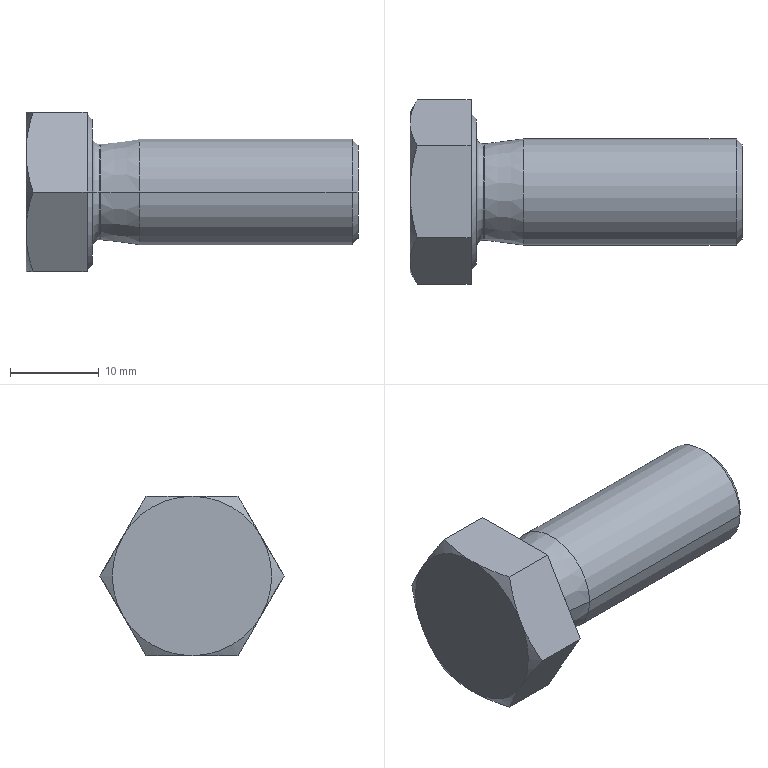Part | SolidWorks | features Chamfer 2, RevCut 2, Revolution 2, Extrusion 1, ICE 1 | 1 solid | 28 faces | box 37.5 x 20.785 x 18 mm | volume 5393 mm3 | cone 12 | plane 10 | torus 4 | cylinder 2 | commonest cylinder face diameters 12 x2
STEP:
#1=CARTESIAN_POINT('',(7.5,-6.282,0.));
#2=VERTEX_POINT('',#1);
#3=CARTESIAN_POINT('',(8.35,-5.432,0.));
#4=VERTEX_POINT('',#3);
#5=CARTESIAN_POINT('',(8.35,-6.282,0.));
#6=DIRECTION('',(0.,0.,-1.));
#7=DIRECTION('',(-1.,0.,0.));
#8=AXIS2_PLACEMENT_3D('',#5,#6,#7);
#9=CIRCLE('',#8,0.85);
#10=EDGE_CURVE('',#2,#4,#9,.T.);
#11=ORIENTED_EDGE('',*,*,#10,.T.);
#12=CARTESIAN_POINT('',(8.35,5.432,0.));
#13=VERTEX_POINT('',#12);
#14=CARTESIAN_POINT('',(8.35,0.,0.));
#15=DIRECTION('',(-1.,0.,0.));
#16=DIRECTION('',(0.,-1.,0.));
#17=AXIS2_PLACEMENT_3D('',#14,#15,#16);
#18=CIRCLE('',#17,5.432);
#19=EDGE_CURVE('',#4,#13,#18,.T.);
#20=ORIENTED_EDGE('',*,*,#19,.T.);
#21=CARTESIAN_POINT('',(7.5,6.282,0.));
#22=VERTEX_POINT('',#21);
#23=CARTESIAN_POINT('',(8.35,6.282,0.));
#24=DIRECTION('',(0.,0.,1.));
#25=DIRECTION('',(0.,-1.,0.));
#26=AXIS2_PLACEMENT_3D('',#23,#24,#25);
#27=CIRCLE('',#26,0.85);
#28=EDGE_CURVE('',#22,#13,#27,.T.);
#29=ORIENTED_EDGE('',*,*,#28,.F.);
#30=CARTESIAN_POINT('',(7.5,0.,0.));
#31=DIRECTION('',(-1.,0.,0.));
#32=DIRECTION('',(0.,-1.,0.));
#33=AXIS2_PLACEMENT_3D('',#30,#31,#32);
#34=CIRCLE('',#33,6.282);
#35=EDGE_CURVE('',#2,#22,#34,.T.);
#36=ORIENTED_EDGE('',*,*,#35,.F.);
#37=EDGE_LOOP('',(#11,#20,#29,#36));
#38=FACE_OUTER_BOUND('',#37,.T.);
#39=CARTESIAN_POINT('',(8.35,0.,0.));
#40=DIRECTION('',(-1.,0.,0.));
#41=DIRECTION('',(0.,-1.,0.));
#42=AXIS2_PLACEMENT_3D('',#39,#40,#41);
#43=TOROIDAL_SURFACE('',#42,6.282,0.85);
#44=ADVANCED_FACE('',(#38),#43,.F.);
#45=ORIENTED_EDGE('',*,*,#28,.T.);
#46=CARTESIAN_POINT('',(8.35,0.,0.));
#47=DIRECTION('',(-1.,0.,0.));
#48=DIRECTION('',(0.,-1.,0.));
#49=AXIS2_PLACEMENT_3D('',#46,#47,#48);
#50=CIRCLE('',#49,5.432);
#51=EDGE_CURVE('',#13,#4,#50,.T.);
#52=ORIENTED_EDGE('',*,*,#51,.T.);
#53=ORIENTED_EDGE('',*,*,#10,.F.);
#54=CARTESIAN_POINT('',(7.5,0.,0.));
#55=DIRECTION('',(-1.,0.,0.));
#56=DIRECTION('',(0.,-1.,0.));
#57=AXIS2_PLACEMENT_3D('',#54,#55,#56);
#58=CIRCLE('',#57,6.282);
#59=EDGE_CURVE('',#22,#2,#58,.T.);
#60=ORIENTED_EDGE('',*,*,#59,.F.);
#61=EDGE_LOOP('',(#45,#52,#53,#60));
#62=FACE_OUTER_BOUND('',#61,.T.);
#63=CARTESIAN_POINT('',(8.35,0.,0.));
#64=DIRECTION('',(-1.,0.,0.));
#65=DIRECTION('',(0.,-1.,0.));
#66=AXIS2_PLACEMENT_3D('',#63,#64,#65);
#67=TOROIDAL_SURFACE('',#66,6.282,0.85);
#68=ADVANCED_FACE('',(#62),#67,.F.);
#69=CARTESIAN_POINT('',(7.5,-8.215,0.));
#70=VERTEX_POINT('',#69);
#71=CARTESIAN_POINT('',(7.5,8.215,0.));
#72=VERTEX_POINT('',#71);
#73=CARTESIAN_POINT('',(7.5,0.,0.));
#74=DIRECTION('',(-1.,0.,0.));
#75=DIRECTION('',(0.,-1.,0.));
#76=AXIS2_PLACEMENT_3D('',#73,#74,#75);
#77=CIRCLE('',#76,8.215);
#78=EDGE_CURVE('',#70,#72,#77,.T.);
#79=ORIENTED_EDGE('',*,*,#78,.T.);
#80=CARTESIAN_POINT('',(6.9,8.815,0.));
#81=VERTEX_POINT('',#80);
#82=CARTESIAN_POINT('',(6.9,8.815,0.));
#83=DIRECTION('',(-0.7071,0.7071,0.));
#84=VECTOR('',#83,1000.);
#85=LINE('',#82,#84);
#86=EDGE_CURVE('',#72,#81,#85,.T.);
#87=ORIENTED_EDGE('',*,*,#86,.T.);
#88=CARTESIAN_POINT('',(6.9,-8.815,0.));
#89=VERTEX_POINT('',#88);
#90=CARTESIAN_POINT('',(6.9,0.,0.));
#91=DIRECTION('',(-1.,0.,0.));
#92=DIRECTION('',(0.,-1.,0.));
#93=AXIS2_PLACEMENT_3D('',#90,#91,#92);
#94=CIRCLE('',#93,8.815);
#95=EDGE_CURVE('',#89,#81,#94,.T.);
#96=ORIENTED_EDGE('',*,*,#95,.F.);
#97=CARTESIAN_POINT('',(6.9,-8.815,0.));
#98=DIRECTION('',(-0.7071,-0.7071,0.));
#99=VECTOR('',#98,1000.);
#100=LINE('',#97,#99);
#101=EDGE_CURVE('',#70,#89,#100,.T.);
#102=ORIENTED_EDGE('',*,*,#101,.F.);
#103=EDGE_LOOP('',(#79,#87,#96,#102));
#104=FACE_OUTER_BOUND('',#103,.T.);
#105=CARTESIAN_POINT('',(6.9,0.,0.));
#106=DIRECTION('',(-1.,0.,0.));
#107=DIRECTION('',(0.,-1.,0.));
#108=AXIS2_PLACEMENT_3D('',#105,#106,#107);
#109=CONICAL_SURFACE('',#108,8.815,0.7854);
#110=ADVANCED_FACE('',(#104),#109,.T.);
#111=CARTESIAN_POINT('',(37.5,5.333,0.));
#112=VERTEX_POINT('',#111);
#113=CARTESIAN_POINT('',(37.5,-5.333,0.));
#114=VERTEX_POINT('',#113);
#115=CARTESIAN_POINT('',(37.5,0.,0.));
#116=DIRECTION('',(1.,0.,0.));
#117=DIRECTION('',(0.,-1.,0.));
#118=AXIS2_PLACEMENT_3D('',#115,#116,#117);
#119=CIRCLE('',#118,5.333);
#120=EDGE_CURVE('',#112,#114,#119,.T.);
#121=ORIENTED_EDGE('',*,*,#120,.F.);
#122=CARTESIAN_POINT('',(36.833,6.,0.));
#123=VERTEX_POINT('',#122);
#124=CARTESIAN_POINT('',(36.833,6.,0.));
#125=DIRECTION('',(-0.7071,0.7071,0.));
#126=VECTOR('',#125,1000.);
#127=LINE('',#124,#126);
#128=EDGE_CURVE('',#112,#123,#127,.T.);
#129=ORIENTED_EDGE('',*,*,#128,.T.);
#130=CARTESIAN_POINT('',(36.833,-6.,0.));
#131=VERTEX_POINT('',#130);
#132=CARTESIAN_POINT('',(36.833,0.,0.));
#133=DIRECTION('',(-1.,0.,0.));
#134=DIRECTION('',(0.,-1.,0.));
#135=AXIS2_PLACEMENT_3D('',#132,#133,#134);
#136=CIRCLE('',#135,6.);
#137=EDGE_CURVE('',#131,#123,#136,.T.);
#138=ORIENTED_EDGE('',*,*,#137,.F.);
#139=CARTESIAN_POINT('',(36.833,-6.,0.));
#140=DIRECTION('',(-0.7071,-0.7071,0.));
#141=VECTOR('',#140,1000.);
#142=LINE('',#139,#141);
#143=EDGE_CURVE('',#114,#131,#142,.T.);
#144=ORIENTED_EDGE('',*,*,#143,.F.);
#145=EDGE_LOOP('',(#121,#129,#138,#144));
#146=FACE_OUTER_BOUND('',#145,.T.);
#147=CARTESIAN_POINT('',(36.833,0.,0.));
#148=DIRECTION('',(-1.,0.,0.));
#149=DIRECTION('',(0.,-1.,0.));
#150=AXIS2_PLACEMENT_3D('',#147,#148,#149);
#151=CONICAL_SURFACE('',#150,6.,0.7854);
#152=ADVANCED_FACE('',(#146),#151,.T.);
#153=ORIENTED_EDGE('',*,*,#51,.F.);
#154=CARTESIAN_POINT('',(8.459,5.439,0.));
#155=VERTEX_POINT('',#154);
#156=CARTESIAN_POINT('',(8.35,6.282,0.));
#157=DIRECTION('',(0.,0.,1.));
#158=DIRECTION('',(0.,-1.,0.));
#159=AXIS2_PLACEMENT_3D('',#156,#157,#158);
#160=CIRCLE('',#159,0.85);
#161=EDGE_CURVE('',#13,#155,#160,.T.);
#162=ORIENTED_EDGE('',*,*,#161,.T.);
#163=CARTESIAN_POINT('',(8.459,-5.439,0.));
#164=VERTEX_POINT('',#163);
#165=CARTESIAN_POINT('',(8.459,0.,0.));
#166=DIRECTION('',(-1.,0.,0.));
#167=DIRECTION('',(0.,-1.,0.));
#168=AXIS2_PLACEMENT_3D('',#165,#166,#167);
#169=CIRCLE('',#168,5.439);
#170=EDGE_CURVE('',#155,#164,#169,.T.);
#171=ORIENTED_EDGE('',*,*,#170,.T.);
#172=CARTESIAN_POINT('',(8.35,-6.282,0.));
#173=DIRECTION('',(0.,0.,-1.));
#174=DIRECTION('',(-1.,0.,0.));
#175=AXIS2_PLACEMENT_3D('',#172,#173,#174);
#176=CIRCLE('',#175,0.85);
#177=EDGE_CURVE('',#4,#164,#176,.T.);
#178=ORIENTED_EDGE('',*,*,#177,.F.);
#179=EDGE_LOOP('',(#153,#162,#171,#178));
#180=FACE_OUTER_BOUND('',#179,.T.);
#181=CARTESIAN_POINT('',(8.35,0.,0.));
#182=DIRECTION('',(-1.,0.,0.));
#183=DIRECTION('',(0.,-1.,0.));
#184=AXIS2_PLACEMENT_3D('',#181,#182,#183);
#185=TOROIDAL_SURFACE('',#184,6.282,0.85);
#186=ADVANCED_FACE('',(#180),#185,.F.);
#187=ORIENTED_EDGE('',*,*,#137,.T.);
#188=CARTESIAN_POINT('',(12.8,6.,0.));
#189=VERTEX_POINT('',#188);
#190=CARTESIAN_POINT('',(7.5,6.,0.));
#191=DIRECTION('',(-1.,0.,0.));
#192=VECTOR('',#191,1000.);
#193=LINE('',#190,#192);
#194=EDGE_CURVE('',#123,#189,#193,.T.);
#195=ORIENTED_EDGE('',*,*,#194,.T.);
#196=CARTESIAN_POINT('',(12.8,-6.,0.));
#197=VERTEX_POINT('',#196);
#198=CARTESIAN_POINT('',(12.8,0.,0.));
#199=DIRECTION('',(-1.,0.,0.));
#200=DIRECTION('',(0.,-1.,0.));
#201=AXIS2_PLACEMENT_3D('',#198,#199,#200);
#202=CIRCLE('',#201,6.);
#203=EDGE_CURVE('',#197,#189,#202,.T.);
#204=ORIENTED_EDGE('',*,*,#203,.F.);
#205=CARTESIAN_POINT('',(7.5,-6.,0.));
#206=DIRECTION('',(-1.,0.,0.));
#207=VECTOR('',#206,1000.);
#208=LINE('',#205,#207);
#209=EDGE_CURVE('',#131,#197,#208,.T.);
#210=ORIENTED_EDGE('',*,*,#209,.F.);
#211=EDGE_LOOP('',(#187,#195,#204,#210));
#212=FACE_OUTER_BOUND('',#211,.T.);
#213=CARTESIAN_POINT('',(7.5,0.,0.));
#214=DIRECTION('',(-1.,0.,0.));
#215=DIRECTION('',(0.,-1.,0.));
#216=AXIS2_PLACEMENT_3D('',#213,#214,#215);
#217=CYLINDRICAL_SURFACE('',#216,6.);
#218=ADVANCED_FACE('',(#212),#217,.T.);
#219=CARTESIAN_POINT('',(8.459,0.,0.));
#220=DIRECTION('',(-1.,0.,0.));
#221=DIRECTION('',(0.,-1.,0.));
#222=AXIS2_PLACEMENT_3D('',#219,#220,#221);
#223=CIRCLE('',#222,5.439);
#224=EDGE_CURVE('',#164,#155,#223,.T.);
#225=ORIENTED_EDGE('',*,*,#224,.F.);
#226=CARTESIAN_POINT('',(12.8,-6.,0.));
#227=DIRECTION('',(0.9917,-0.1282,0.));
#228=VECTOR('',#227,1000.);
#229=LINE('',#226,#228);
#230=EDGE_CURVE('',#164,#197,#229,.T.);
#231=ORIENTED_EDGE('',*,*,#230,.T.);
#232=ORIENTED_EDGE('',*,*,#203,.T.);
#233=CARTESIAN_POINT('',(12.8,6.,0.));
#234=DIRECTION('',(0.9917,0.1282,0.));
#235=VECTOR('',#234,1000.);
#236=LINE('',#233,#235);
#237=EDGE_CURVE('',#155,#189,#236,.T.);
#238=ORIENTED_EDGE('',*,*,#237,.F.);
#239=EDGE_LOOP('',(#225,#231,#232,#238));
#240=FACE_OUTER_BOUND('',#239,.T.);
#241=CARTESIAN_POINT('',(12.8,0.,0.));
#242=DIRECTION('',(1.,0.,0.));
#243=DIRECTION('',(0.,1.,0.));
#244=AXIS2_PLACEMENT_3D('',#241,#242,#243);
#245=CONICAL_SURFACE('',#244,6.,0.1286);
#246=ADVANCED_FACE('',(#240),#245,.T.);
#247=ORIENTED_EDGE('',*,*,#35,.T.);
#248=ORIENTED_EDGE('',*,*,#59,.T.);
#249=EDGE_LOOP('',(#247,#248));
#250=FACE_BOUND('',#249,.T.);
#251=ORIENTED_EDGE('',*,*,#78,.F.);
#252=CARTESIAN_POINT('',(7.5,0.,0.));
#253=DIRECTION('',(-1.,0.,0.));
#254=DIRECTION('',(0.,-1.,0.));
#255=AXIS2_PLACEMENT_3D('',#252,#253,#254);
#256=CIRCLE('',#255,8.215);
#257=EDGE_CURVE('',#72,#70,#256,.T.);
#258=ORIENTED_EDGE('',*,*,#257,.F.);
#259=EDGE_LOOP('',(#251,#258));
#260=FACE_OUTER_BOUND('',#259,.T.);
#261=CARTESIAN_POINT('',(7.5,5.196,-9.));
#262=DIRECTION('',(1.,0.,0.));
#263=DIRECTION('',(0.,0.,-1.));
#264=AXIS2_PLACEMENT_3D('',#261,#262,#263);
#265=PLANE('',#264);
#266=ADVANCED_FACE('',(#250,#260),#265,.T.);
#267=ORIENTED_EDGE('',*,*,#230,.F.);
#268=ORIENTED_EDGE('',*,*,#170,.F.);
#269=ORIENTED_EDGE('',*,*,#237,.T.);
#270=CARTESIAN_POINT('',(12.8,0.,0.));
#271=DIRECTION('',(-1.,0.,0.));
#272=DIRECTION('',(0.,-1.,0.));
#273=AXIS2_PLACEMENT_3D('',#270,#271,#272);
#274=CIRCLE('',#273,6.);
#275=EDGE_CURVE('',#189,#197,#274,.T.);
#276=ORIENTED_EDGE('',*,*,#275,.T.);
#277=EDGE_LOOP('',(#267,#268,#269,#276));
#278=FACE_OUTER_BOUND('',#277,.T.);
#279=CARTESIAN_POINT('',(12.8,0.,0.));
#280=DIRECTION('',(1.,0.,0.));
#281=DIRECTION('',(0.,1.,0.));
#282=AXIS2_PLACEMENT_3D('',#279,#280,#281);
#283=CONICAL_SURFACE('',#282,6.,0.1286);
#284=ADVANCED_FACE('',(#278),#283,.T.);
#285=ORIENTED_EDGE('',*,*,#194,.F.);
#286=CARTESIAN_POINT('',(36.833,0.,0.));
#287=DIRECTION('',(-1.,0.,0.));
#288=DIRECTION('',(0.,-1.,0.));
#289=AXIS2_PLACEMENT_3D('',#286,#287,#288);
#290=CIRCLE('',#289,6.);
#291=EDGE_CURVE('',#123,#131,#290,.T.);
#292=ORIENTED_EDGE('',*,*,#291,.T.);
#293=ORIENTED_EDGE('',*,*,#209,.T.);
#294=ORIENTED_EDGE('',*,*,#275,.F.);
#295=EDGE_LOOP('',(#285,#292,#293,#294));
#296=FACE_OUTER_BOUND('',#295,.T.);
#297=CARTESIAN_POINT('',(7.5,0.,0.));
#298=DIRECTION('',(-1.,0.,0.));
#299=DIRECTION('',(0.,-1.,0.));
#300=AXIS2_PLACEMENT_3D('',#297,#298,#299);
#301=CYLINDRICAL_SURFACE('',#300,6.);
#302=ADVANCED_FACE('',(#296),#301,.T.);
#303=CARTESIAN_POINT('',(37.5,0.,0.));
#304=DIRECTION('',(1.,0.,0.));
#305=DIRECTION('',(0.,-1.,0.));
#306=AXIS2_PLACEMENT_3D('',#303,#304,#305);
#307=CIRCLE('',#306,5.333);
#308=EDGE_CURVE('',#114,#112,#307,.T.);
#309=ORIENTED_EDGE('',*,*,#308,.T.);
#310=ORIENTED_EDGE('',*,*,#120,.T.);
#311=EDGE_LOOP('',(#309,#310));
#312=FACE_OUTER_BOUND('',#311,.T.);
#313=CARTESIAN_POINT('',(37.5,6.,0.));
#314=DIRECTION('',(-1.,0.,0.));
#315=DIRECTION('',(0.,-1.,0.));
#316=AXIS2_PLACEMENT_3D('',#313,#314,#315);
#317=PLANE('',#316);
#318=ADVANCED_FACE('',(#312),#317,.F.);
#319=ORIENTED_EDGE('',*,*,#19,.F.);
#320=ORIENTED_EDGE('',*,*,#177,.T.);
#321=ORIENTED_EDGE('',*,*,#224,.T.);
#322=ORIENTED_EDGE('',*,*,#161,.F.);
#323=EDGE_LOOP('',(#319,#320,#321,#322));
#324=FACE_OUTER_BOUND('',#323,.T.);
#325=CARTESIAN_POINT('',(8.35,0.,0.));
#326=DIRECTION('',(-1.,0.,0.));
#327=DIRECTION('',(0.,-1.,0.));
#328=AXIS2_PLACEMENT_3D('',#325,#326,#327);
#329=TOROIDAL_SURFACE('',#328,6.282,0.85);
#330=ADVANCED_FACE('',(#324),#329,.F.);
#331=ORIENTED_EDGE('',*,*,#128,.F.);
#332=ORIENTED_EDGE('',*,*,#308,.F.);
#333=ORIENTED_EDGE('',*,*,#143,.T.);
#334=ORIENTED_EDGE('',*,*,#291,.F.);
#335=EDGE_LOOP('',(#331,#332,#333,#334));
#336=FACE_OUTER_BOUND('',#335,.T.);
#337=CARTESIAN_POINT('',(36.833,0.,0.));
#338=DIRECTION('',(-1.,0.,0.));
#339=DIRECTION('',(0.,-1.,0.));
#340=AXIS2_PLACEMENT_3D('',#337,#338,#339);
#341=CONICAL_SURFACE('',#340,6.,0.7854);
#342=ADVANCED_FACE('',(#336),#341,.T.);
#343=ORIENTED_EDGE('',*,*,#95,.T.);
#344=CARTESIAN_POINT('',(6.9,0.,0.));
#345=DIRECTION('',(-1.,0.,0.));
#346=DIRECTION('',(0.,-1.,0.));
#347=AXIS2_PLACEMENT_3D('',#344,#345,#346);
#348=CIRCLE('',#347,8.815);
#349=EDGE_CURVE('',#81,#89,#348,.T.);
#350=ORIENTED_EDGE('',*,*,#349,.T.);
#351=EDGE_LOOP('',(#343,#350));
#352=FACE_BOUND('',#351,.T.);
#353=CARTESIAN_POINT('',(6.9,-5.196,-9.));
#354=VERTEX_POINT('',#353);
#355=CARTESIAN_POINT('',(6.9,5.196,-9.));
#356=VERTEX_POINT('',#355);
#357=CARTESIAN_POINT('',(6.9,-5.196,-9.));
#358=DIRECTION('',(0.,1.,0.));
#359=VECTOR('',#358,1000.);
#360=LINE('',#357,#359);
#361=EDGE_CURVE('',#354,#356,#360,.T.);
#362=ORIENTED_EDGE('',*,*,#361,.T.);
#363=CARTESIAN_POINT('',(6.9,10.392,0.));
#364=VERTEX_POINT('',#363);
#365=CARTESIAN_POINT('',(6.9,5.196,-9.));
#366=DIRECTION('',(0.,0.5,0.866));
#367=VECTOR('',#366,1000.);
#368=LINE('',#365,#367);
#369=EDGE_CURVE('',#356,#364,#368,.T.);
#370=ORIENTED_EDGE('',*,*,#369,.T.);
#371=CARTESIAN_POINT('',(6.9,5.196,9.));
#372=VERTEX_POINT('',#371);
#373=CARTESIAN_POINT('',(6.9,10.392,0.));
#374=DIRECTION('',(0.,-0.5,0.866));
#375=VECTOR('',#374,1000.);
#376=LINE('',#373,#375);
#377=EDGE_CURVE('',#364,#372,#376,.T.);
#378=ORIENTED_EDGE('',*,*,#377,.T.);
#379=CARTESIAN_POINT('',(6.9,-5.196,9.));
#380=VERTEX_POINT('',#379);
#381=CARTESIAN_POINT('',(6.9,5.196,9.));
#382=DIRECTION('',(0.,-1.,0.));
#383=VECTOR('',#382,1000.);
#384=LINE('',#381,#383);
#385=EDGE_CURVE('',#372,#380,#384,.T.);
#386=ORIENTED_EDGE('',*,*,#385,.T.);
#387=CARTESIAN_POINT('',(6.9,-10.392,0.));
#388=VERTEX_POINT('',#387);
#389=CARTESIAN_POINT('',(6.9,-5.196,9.));
#390=DIRECTION('',(0.,-0.5,-0.866));
#391=VECTOR('',#390,1000.);
#392=LINE('',#389,#391);
#393=EDGE_CURVE('',#380,#388,#392,.T.);
#394=ORIENTED_EDGE('',*,*,#393,.T.);
#395=CARTESIAN_POINT('',(6.9,-10.392,0.));
#396=DIRECTION('',(0.,0.5,-0.866));
#397=VECTOR('',#396,1000.);
#398=LINE('',#395,#397);
#399=EDGE_CURVE('',#388,#354,#398,.T.);
#400=ORIENTED_EDGE('',*,*,#399,.T.);
#401=EDGE_LOOP('',(#362,#370,#378,#386,#394,#400));
#402=FACE_OUTER_BOUND('',#401,.T.);
#403=CARTESIAN_POINT('',(6.9,-8.815,0.));
#404=DIRECTION('',(1.,0.,0.));
#405=DIRECTION('',(0.,1.,0.));
#406=AXIS2_PLACEMENT_3D('',#403,#404,#405);
#407=PLANE('',#406);
#408=ADVANCED_FACE('',(#352,#402),#407,.T.);
#409=ORIENTED_EDGE('',*,*,#86,.F.);
#410=ORIENTED_EDGE('',*,*,#257,.T.);
#411=ORIENTED_EDGE('',*,*,#101,.T.);
#412=ORIENTED_EDGE('',*,*,#349,.F.);
#413=EDGE_LOOP('',(#409,#410,#411,#412));
#414=FACE_OUTER_BOUND('',#413,.T.);
#415=CARTESIAN_POINT('',(6.9,0.,0.));
#416=DIRECTION('',(-1.,0.,0.));
#417=DIRECTION('',(0.,-1.,0.));
#418=AXIS2_PLACEMENT_3D('',#415,#416,#417);
#419=CONICAL_SURFACE('',#418,8.815,0.7854);
#420=ADVANCED_FACE('',(#414),#419,.T.);
#421=CARTESIAN_POINT('',(0.,0.,-9.));
#422=VERTEX_POINT('',#421);
#423=CARTESIAN_POINT('',(0.,7.794,-4.5));
#424=VERTEX_POINT('',#423);
#425=CARTESIAN_POINT('',(0.,0.,0.));
#426=DIRECTION('',(1.,0.,0.));
#427=DIRECTION('',(0.,0.,-1.));
#428=AXIS2_PLACEMENT_3D('',#425,#426,#427);
#429=CIRCLE('',#428,9.);
#430=EDGE_CURVE('',#422,#424,#429,.T.);
#431=ORIENTED_EDGE('',*,*,#430,.F.);
#432=CARTESIAN_POINT('',(0.,-7.794,-4.5));
#433=VERTEX_POINT('',#432);
#434=CARTESIAN_POINT('',(0.,0.,0.));
#435=DIRECTION('',(1.,0.,0.));
#436=DIRECTION('',(0.,0.,-1.));
#437=AXIS2_PLACEMENT_3D('',#434,#435,#436);
#438=CIRCLE('',#437,9.);
#439=EDGE_CURVE('',#433,#422,#438,.T.);
#440=ORIENTED_EDGE('',*,*,#439,.F.);
#441=CARTESIAN_POINT('',(0.,-7.794,4.5));
#442=VERTEX_POINT('',#441);
#443=CARTESIAN_POINT('',(0.,0.,0.));
#444=DIRECTION('',(1.,0.,0.));
#445=DIRECTION('',(0.,0.,-1.));
#446=AXIS2_PLACEMENT_3D('',#443,#444,#445);
#447=CIRCLE('',#446,9.);
#448=EDGE_CURVE('',#442,#433,#447,.T.);
#449=ORIENTED_EDGE('',*,*,#448,.F.);
#450=CARTESIAN_POINT('',(0.,0.,9.));
#451=VERTEX_POINT('',#450);
#452=CARTESIAN_POINT('',(0.,0.,0.));
#453=DIRECTION('',(1.,0.,0.));
#454=DIRECTION('',(0.,0.,-1.));
#455=AXIS2_PLACEMENT_3D('',#452,#453,#454);
#456=CIRCLE('',#455,9.);
#457=EDGE_CURVE('',#451,#442,#456,.T.);
#458=ORIENTED_EDGE('',*,*,#457,.F.);
#459=CARTESIAN_POINT('',(0.,7.794,4.5));
#460=VERTEX_POINT('',#459);
#461=CARTESIAN_POINT('',(0.,0.,0.));
#462=DIRECTION('',(-1.,0.,0.));
#463=DIRECTION('',(0.,0.,1.));
#464=AXIS2_PLACEMENT_3D('',#461,#462,#463);
#465=CIRCLE('',#464,9.);
#466=EDGE_CURVE('',#451,#460,#465,.T.);
#467=ORIENTED_EDGE('',*,*,#466,.T.);
#468=CARTESIAN_POINT('',(0.,0.,0.));
#469=DIRECTION('',(1.,0.,0.));
#470=DIRECTION('',(0.,0.,-1.));
#471=AXIS2_PLACEMENT_3D('',#468,#469,#470);
#472=CIRCLE('',#471,9.);
#473=EDGE_CURVE('',#424,#460,#472,.T.);
#474=ORIENTED_EDGE('',*,*,#473,.F.);
#475=EDGE_LOOP('',(#431,#440,#449,#458,#467,#474));
#476=FACE_OUTER_BOUND('',#475,.T.);
#477=CARTESIAN_POINT('',(0.,5.196,-9.));
#478=DIRECTION('',(1.,0.,0.));
#479=DIRECTION('',(0.,0.,-1.));
#480=AXIS2_PLACEMENT_3D('',#477,#478,#479);
#481=PLANE('',#480);
#482=ADVANCED_FACE('',(#476),#481,.F.);
#483=CARTESIAN_POINT('',(0.8038,5.196,-9.));
#484=VERTEX_POINT('',#483);
#485=CARTESIAN_POINT('',(0.,7.794,-4.5));
#486=CARTESIAN_POINT('',(0.,7.574,-4.882));
#487=CARTESIAN_POINT('',(0.019,7.352,-5.266));
#488=CARTESIAN_POINT('',(0.09253,6.914,-6.024));
#489=CARTESIAN_POINT('',(0.147,6.697,-6.401));
#490=CARTESIAN_POINT('',(0.357,6.048,-7.525));
#491=CARTESIAN_POINT('',(0.5591,5.62,-8.266));
#492=CARTESIAN_POINT('',(0.8038,5.196,-9.));
#493=B_SPLINE_CURVE_WITH_KNOTS('',3,(#485,#486,#487,#488,#489,#490,#491,#492),.UNSPECIFIED.,.F.,.F.,(4,2,2,4),(0.005258,0.006567,0.007877,0.0105),.UNSPECIFIED.);
#494=EDGE_CURVE('',#424,#484,#493,.T.);
#495=ORIENTED_EDGE('',*,*,#494,.T.);
#496=CARTESIAN_POINT('',(0.8038,5.196,-9.));
#497=CARTESIAN_POINT('',(0.5613,4.356,-9.));
#498=CARTESIAN_POINT('',(0.3593,3.505,-9.));
#499=CARTESIAN_POINT('',(0.07758,1.769,-9.));
#500=CARTESIAN_POINT('',(0.,0.8787,-9.));
#501=CARTESIAN_POINT('',(0.,0.,-9.));
#502=B_SPLINE_CURVE_WITH_KNOTS('',3,(#496,#497,#498,#499,#500,#501),.UNSPECIFIED.,.F.,.F.,(4,2,4),(0.003787,0.00641,0.009033),.UNSPECIFIED.);
#503=EDGE_CURVE('',#484,#422,#502,.T.);
#504=ORIENTED_EDGE('',*,*,#503,.T.);
#505=ORIENTED_EDGE('',*,*,#430,.T.);
#506=EDGE_LOOP('',(#495,#504,#505));
#507=FACE_OUTER_BOUND('',#506,.T.);
#508=CARTESIAN_POINT('',(0.,0.,0.));
#509=DIRECTION('',(1.,0.,0.));
#510=DIRECTION('',(0.,0.,1.));
#511=AXIS2_PLACEMENT_3D('',#508,#509,#510);
#512=CONICAL_SURFACE('',#511,9.,1.047);
#513=ADVANCED_FACE('',(#507),#512,.T.);
#514=CARTESIAN_POINT('',(0.8038,10.392,0.));
#515=VERTEX_POINT('',#514);
#516=CARTESIAN_POINT('',(0.,7.794,4.5));
#517=CARTESIAN_POINT('',(0.,8.015,4.118));
#518=CARTESIAN_POINT('',(0.019,8.236,3.734));
#519=CARTESIAN_POINT('',(0.09253,8.674,2.976));
#520=CARTESIAN_POINT('',(0.147,8.892,2.599));
#521=CARTESIAN_POINT('',(0.357,9.541,1.475));
#522=CARTESIAN_POINT('',(0.5591,9.968,0.7343));
#523=CARTESIAN_POINT('',(0.8038,10.392,0.));
#524=B_SPLINE_CURVE_WITH_KNOTS('',3,(#516,#517,#518,#519,#520,#521,#522,#523),.UNSPECIFIED.,.F.,.F.,(4,2,2,4),(0.005258,0.006567,0.007877,0.0105),.UNSPECIFIED.);
#525=EDGE_CURVE('',#460,#515,#524,.T.);
#526=ORIENTED_EDGE('',*,*,#525,.T.);
#527=CARTESIAN_POINT('',(0.8038,10.392,0.));
#528=CARTESIAN_POINT('',(0.5585,9.967,-0.7361));
#529=CARTESIAN_POINT('',(0.3563,9.539,-1.478));
#530=CARTESIAN_POINT('',(0.07661,8.674,-2.976));
#531=CARTESIAN_POINT('',(0.,8.237,-3.733));
#532=CARTESIAN_POINT('',(0.,7.794,-4.5));
#533=B_SPLINE_CURVE_WITH_KNOTS('',3,(#527,#528,#529,#530,#531,#532),.UNSPECIFIED.,.F.,.F.,(4,2,4),(0.000000238,0.002629,0.005258),.UNSPECIFIED.);
#534=EDGE_CURVE('',#515,#424,#533,.T.);
#535=ORIENTED_EDGE('',*,*,#534,.T.);
#536=ORIENTED_EDGE('',*,*,#473,.T.);
#537=EDGE_LOOP('',(#526,#535,#536));
#538=FACE_OUTER_BOUND('',#537,.T.);
#539=CARTESIAN_POINT('',(0.,0.,0.));
#540=DIRECTION('',(1.,0.,0.));
#541=DIRECTION('',(0.,0.,1.));
#542=AXIS2_PLACEMENT_3D('',#539,#540,#541);
#543=CONICAL_SURFACE('',#542,9.,1.047);
#544=ADVANCED_FACE('',(#538),#543,.T.);
#545=CARTESIAN_POINT('',(0.8038,5.196,9.));
#546=VERTEX_POINT('',#545);
#547=CARTESIAN_POINT('',(0.8038,5.196,9.));
#548=CARTESIAN_POINT('',(0.5585,5.621,8.264));
#549=CARTESIAN_POINT('',(0.3563,6.049,7.522));
#550=CARTESIAN_POINT('',(0.07661,6.914,6.024));
#551=CARTESIAN_POINT('',(0.,7.352,5.267));
#552=CARTESIAN_POINT('',(0.,7.794,4.5));
#553=B_SPLINE_CURVE_WITH_KNOTS('',3,(#547,#548,#549,#550,#551,#552),.UNSPECIFIED.,.F.,.F.,(4,2,4),(0.000000238,0.002629,0.005258),.UNSPECIFIED.);
#554=EDGE_CURVE('',#546,#460,#553,.T.);
#555=ORIENTED_EDGE('',*,*,#554,.T.);
#556=ORIENTED_EDGE('',*,*,#466,.F.);
#557=CARTESIAN_POINT('',(0.,0.,9.));
#558=CARTESIAN_POINT('',(0.,0.8787,9.));
#559=CARTESIAN_POINT('',(0.07758,1.769,9.));
#560=CARTESIAN_POINT('',(0.3593,3.505,9.));
#561=CARTESIAN_POINT('',(0.5613,4.356,9.));
#562=CARTESIAN_POINT('',(0.8038,5.196,9.));
#563=B_SPLINE_CURVE_WITH_KNOTS('',3,(#557,#558,#559,#560,#561,#562),.UNSPECIFIED.,.F.,.F.,(4,2,4),(0.01455,0.01718,0.01981),.UNSPECIFIED.);
#564=EDGE_CURVE('',#451,#546,#563,.T.);
#565=ORIENTED_EDGE('',*,*,#564,.T.);
#566=EDGE_LOOP('',(#555,#556,#565));
#567=FACE_OUTER_BOUND('',#566,.T.);
#568=CARTESIAN_POINT('',(0.,0.,0.));
#569=DIRECTION('',(1.,0.,0.));
#570=DIRECTION('',(0.,0.,1.));
#571=AXIS2_PLACEMENT_3D('',#568,#569,#570);
#572=CONICAL_SURFACE('',#571,9.,1.047);
#573=ADVANCED_FACE('',(#567),#572,.T.);
#574=CARTESIAN_POINT('',(0.8038,-5.196,9.));
#575=VERTEX_POINT('',#574);
#576=CARTESIAN_POINT('',(0.8038,-5.196,9.));
#577=CARTESIAN_POINT('',(0.5599,-4.351,9.));
#578=CARTESIAN_POINT('',(0.3553,-3.485,9.));
#579=CARTESIAN_POINT('',(0.07548,-1.75,9.));
#580=CARTESIAN_POINT('',(0.,-0.8781,9.));
#581=CARTESIAN_POINT('',(0.,0.,9.));
#582=B_SPLINE_CURVE_WITH_KNOTS('',3,(#576,#577,#578,#579,#580,#581),.UNSPECIFIED.,.F.,.F.,(4,2,4),(0.009291,0.01192,0.01455),.UNSPECIFIED.);
#583=EDGE_CURVE('',#575,#451,#582,.T.);
#584=ORIENTED_EDGE('',*,*,#583,.T.);
#585=ORIENTED_EDGE('',*,*,#457,.T.);
#586=CARTESIAN_POINT('',(0.,-7.794,4.5));
#587=CARTESIAN_POINT('',(0.,-7.574,4.882));
#588=CARTESIAN_POINT('',(0.019,-7.352,5.266));
#589=CARTESIAN_POINT('',(0.09253,-6.914,6.024));
#590=CARTESIAN_POINT('',(0.147,-6.697,6.401));
#591=CARTESIAN_POINT('',(0.357,-6.048,7.525));
#592=CARTESIAN_POINT('',(0.5591,-5.62,8.266));
#593=CARTESIAN_POINT('',(0.8038,-5.196,9.));
#594=B_SPLINE_CURVE_WITH_KNOTS('',3,(#586,#587,#588,#589,#590,#591,#592,#593),.UNSPECIFIED.,.F.,.F.,(4,2,2,4),(0.005258,0.006567,0.007877,0.0105),.UNSPECIFIED.);
#595=EDGE_CURVE('',#442,#575,#594,.T.);
#596=ORIENTED_EDGE('',*,*,#595,.T.);
#597=EDGE_LOOP('',(#584,#585,#596));
#598=FACE_OUTER_BOUND('',#597,.T.);
#599=CARTESIAN_POINT('',(0.,0.,0.));
#600=DIRECTION('',(1.,0.,0.));
#601=DIRECTION('',(0.,0.,1.));
#602=AXIS2_PLACEMENT_3D('',#599,#600,#601);
#603=CONICAL_SURFACE('',#602,9.,1.047);
#604=ADVANCED_FACE('',(#598),#603,.T.);
#605=CARTESIAN_POINT('',(0.8038,-5.196,-9.));
#606=VERTEX_POINT('',#605);
#607=CARTESIAN_POINT('',(0.,0.,-9.));
#608=CARTESIAN_POINT('',(0.,-0.8781,-9.));
#609=CARTESIAN_POINT('',(0.07548,-1.75,-9.));
#610=CARTESIAN_POINT('',(0.3553,-3.485,-9.));
#611=CARTESIAN_POINT('',(0.5599,-4.351,-9.));
#612=CARTESIAN_POINT('',(0.8038,-5.196,-9.));
#613=B_SPLINE_CURVE_WITH_KNOTS('',3,(#607,#608,#609,#610,#611,#612),.UNSPECIFIED.,.F.,.F.,(4,2,4),(0.009033,0.01165,0.01428),.UNSPECIFIED.);
#614=EDGE_CURVE('',#422,#606,#613,.T.);
#615=ORIENTED_EDGE('',*,*,#614,.T.);
#616=CARTESIAN_POINT('',(0.8038,-5.196,-9.));
#617=CARTESIAN_POINT('',(0.5585,-5.621,-8.264));
#618=CARTESIAN_POINT('',(0.3563,-6.049,-7.522));
#619=CARTESIAN_POINT('',(0.07661,-6.914,-6.024));
#620=CARTESIAN_POINT('',(0.,-7.352,-5.267));
#621=CARTESIAN_POINT('',(0.,-7.794,-4.5));
#622=B_SPLINE_CURVE_WITH_KNOTS('',3,(#616,#617,#618,#619,#620,#621),.UNSPECIFIED.,.F.,.F.,(4,2,4),(0.000000238,0.002629,0.005258),.UNSPECIFIED.);
#623=EDGE_CURVE('',#606,#433,#622,.T.);
#624=ORIENTED_EDGE('',*,*,#623,.T.);
#625=ORIENTED_EDGE('',*,*,#439,.T.);
#626=EDGE_LOOP('',(#615,#624,#625));
#627=FACE_OUTER_BOUND('',#626,.T.);
#628=CARTESIAN_POINT('',(0.,0.,0.));
#629=DIRECTION('',(1.,0.,0.));
#630=DIRECTION('',(0.,0.,1.));
#631=AXIS2_PLACEMENT_3D('',#628,#629,#630);
#632=CONICAL_SURFACE('',#631,9.,1.047);
#633=ADVANCED_FACE('',(#627),#632,.T.);
#634=CARTESIAN_POINT('',(0.8038,-10.392,0.));
#635=VERTEX_POINT('',#634);
#636=CARTESIAN_POINT('',(0.8038,-10.392,0.));
#637=CARTESIAN_POINT('',(0.5585,-9.967,0.7361));
#638=CARTESIAN_POINT('',(0.3563,-9.539,1.478));
#639=CARTESIAN_POINT('',(0.07661,-8.674,2.976));
#640=CARTESIAN_POINT('',(0.,-8.237,3.733));
#641=CARTESIAN_POINT('',(0.,-7.794,4.5));
#642=B_SPLINE_CURVE_WITH_KNOTS('',3,(#636,#637,#638,#639,#640,#641),.UNSPECIFIED.,.F.,.F.,(4,2,4),(0.000000238,0.002629,0.005258),.UNSPECIFIED.);
#643=EDGE_CURVE('',#635,#442,#642,.T.);
#644=ORIENTED_EDGE('',*,*,#643,.T.);
#645=ORIENTED_EDGE('',*,*,#448,.T.);
#646=CARTESIAN_POINT('',(0.,-7.794,-4.5));
#647=CARTESIAN_POINT('',(0.,-8.015,-4.118));
#648=CARTESIAN_POINT('',(0.019,-8.236,-3.734));
#649=CARTESIAN_POINT('',(0.09253,-8.674,-2.976));
#650=CARTESIAN_POINT('',(0.147,-8.892,-2.599));
#651=CARTESIAN_POINT('',(0.357,-9.541,-1.475));
#652=CARTESIAN_POINT('',(0.5591,-9.968,-0.7343));
#653=CARTESIAN_POINT('',(0.8038,-10.392,0.));
#654=B_SPLINE_CURVE_WITH_KNOTS('',3,(#646,#647,#648,#649,#650,#651,#652,#653),.UNSPECIFIED.,.F.,.F.,(4,2,2,4),(0.005258,0.006567,0.007877,0.0105),.UNSPECIFIED.);
#655=EDGE_CURVE('',#433,#635,#654,.T.);
#656=ORIENTED_EDGE('',*,*,#655,.T.);
#657=EDGE_LOOP('',(#644,#645,#656));
#658=FACE_OUTER_BOUND('',#657,.T.);
#659=CARTESIAN_POINT('',(0.,0.,0.));
#660=DIRECTION('',(1.,0.,0.));
#661=DIRECTION('',(0.,0.,1.));
#662=AXIS2_PLACEMENT_3D('',#659,#660,#661);
#663=CONICAL_SURFACE('',#662,9.,1.047);
#664=ADVANCED_FACE('',(#658),#663,.T.);
#665=ORIENTED_EDGE('',*,*,#399,.F.);
#666=CARTESIAN_POINT('',(7.5,-10.392,0.));
#667=DIRECTION('',(-1.,0.,0.));
#668=VECTOR('',#667,1000.);
#669=LINE('',#666,#668);
#670=EDGE_CURVE('',#388,#635,#669,.T.);
#671=ORIENTED_EDGE('',*,*,#670,.T.);
#672=ORIENTED_EDGE('',*,*,#655,.F.);
#673=ORIENTED_EDGE('',*,*,#623,.F.);
#674=CARTESIAN_POINT('',(7.5,-5.196,-9.));
#675=DIRECTION('',(-1.,0.,0.));
#676=VECTOR('',#675,1000.);
#677=LINE('',#674,#676);
#678=EDGE_CURVE('',#354,#606,#677,.T.);
#679=ORIENTED_EDGE('',*,*,#678,.F.);
#680=EDGE_LOOP('',(#665,#671,#672,#673,#679));
#681=FACE_OUTER_BOUND('',#680,.T.);
#682=CARTESIAN_POINT('',(7.5,-10.392,0.));
#683=DIRECTION('',(0.,0.866,0.5));
#684=DIRECTION('',(0.,-0.5,0.866));
#685=AXIS2_PLACEMENT_3D('',#682,#683,#684);
#686=PLANE('',#685);
#687=ADVANCED_FACE('',(#681),#686,.F.);
#688=ORIENTED_EDGE('',*,*,#393,.F.);
#689=CARTESIAN_POINT('',(7.5,-5.196,9.));
#690=DIRECTION('',(-1.,0.,0.));
#691=VECTOR('',#690,1000.);
#692=LINE('',#689,#691);
#693=EDGE_CURVE('',#380,#575,#692,.T.);
#694=ORIENTED_EDGE('',*,*,#693,.T.);
#695=ORIENTED_EDGE('',*,*,#595,.F.);
#696=ORIENTED_EDGE('',*,*,#643,.F.);
#697=ORIENTED_EDGE('',*,*,#670,.F.);
#698=EDGE_LOOP('',(#688,#694,#695,#696,#697));
#699=FACE_OUTER_BOUND('',#698,.T.);
#700=CARTESIAN_POINT('',(7.5,-5.196,9.));
#701=DIRECTION('',(0.,0.866,-0.5));
#702=DIRECTION('',(0.,0.5,0.866));
#703=AXIS2_PLACEMENT_3D('',#700,#701,#702);
#704=PLANE('',#703);
#705=ADVANCED_FACE('',(#699),#704,.F.);
#706=ORIENTED_EDGE('',*,*,#385,.F.);
#707=CARTESIAN_POINT('',(7.5,5.196,9.));
#708=DIRECTION('',(-1.,0.,0.));
#709=VECTOR('',#708,1000.);
#710=LINE('',#707,#709);
#711=EDGE_CURVE('',#372,#546,#710,.T.);
#712=ORIENTED_EDGE('',*,*,#711,.T.);
#713=ORIENTED_EDGE('',*,*,#564,.F.);
#714=ORIENTED_EDGE('',*,*,#583,.F.);
#715=ORIENTED_EDGE('',*,*,#693,.F.);
#716=EDGE_LOOP('',(#706,#712,#713,#714,#715));
#717=FACE_OUTER_BOUND('',#716,.T.);
#718=CARTESIAN_POINT('',(7.5,5.196,9.));
#719=DIRECTION('',(0.,0.,-1.));
#720=DIRECTION('',(0.,1.,0.));
#721=AXIS2_PLACEMENT_3D('',#718,#719,#720);
#722=PLANE('',#721);
#723=ADVANCED_FACE('',(#717),#722,.F.);
#724=ORIENTED_EDGE('',*,*,#377,.F.);
#725=CARTESIAN_POINT('',(7.5,10.392,0.));
#726=DIRECTION('',(-1.,0.,0.));
#727=VECTOR('',#726,1000.);
#728=LINE('',#725,#727);
#729=EDGE_CURVE('',#364,#515,#728,.T.);
#730=ORIENTED_EDGE('',*,*,#729,.T.);
#731=ORIENTED_EDGE('',*,*,#525,.F.);
#732=ORIENTED_EDGE('',*,*,#554,.F.);
#733=ORIENTED_EDGE('',*,*,#711,.F.);
#734=EDGE_LOOP('',(#724,#730,#731,#732,#733));
#735=FACE_OUTER_BOUND('',#734,.T.);
#736=CARTESIAN_POINT('',(7.5,10.392,0.));
#737=DIRECTION('',(0.,-0.866,-0.5));
#738=DIRECTION('',(0.,0.5,-0.866));
#739=AXIS2_PLACEMENT_3D('',#736,#737,#738);
#740=PLANE('',#739);
#741=ADVANCED_FACE('',(#735),#740,.F.);
#742=ORIENTED_EDGE('',*,*,#369,.F.);
#743=CARTESIAN_POINT('',(7.5,5.196,-9.));
#744=DIRECTION('',(-1.,0.,0.));
#745=VECTOR('',#744,1000.);
#746=LINE('',#743,#745);
#747=EDGE_CURVE('',#356,#484,#746,.T.);
#748=ORIENTED_EDGE('',*,*,#747,.T.);
#749=ORIENTED_EDGE('',*,*,#494,.F.);
#750=ORIENTED_EDGE('',*,*,#534,.F.);
#751=ORIENTED_EDGE('',*,*,#729,.F.);
#752=EDGE_LOOP('',(#742,#748,#749,#750,#751));
#753=FACE_OUTER_BOUND('',#752,.T.);
#754=CARTESIAN_POINT('',(7.5,5.196,-9.));
#755=DIRECTION('',(0.,-0.866,0.5));
#756=DIRECTION('',(0.,-0.5,-0.866));
#757=AXIS2_PLACEMENT_3D('',#754,#755,#756);
#758=PLANE('',#757);
#759=ADVANCED_FACE('',(#753),#758,.F.);
#760=ORIENTED_EDGE('',*,*,#361,.F.);
#761=ORIENTED_EDGE('',*,*,#678,.T.);
#762=ORIENTED_EDGE('',*,*,#614,.F.);
#763=ORIENTED_EDGE('',*,*,#503,.F.);
#764=ORIENTED_EDGE('',*,*,#747,.F.);
#765=EDGE_LOOP('',(#760,#761,#762,#763,#764));
#766=FACE_OUTER_BOUND('',#765,.T.);
#767=CARTESIAN_POINT('',(7.5,-5.196,-9.));
#768=DIRECTION('',(0.,0.,1.));
#769=DIRECTION('',(0.,-1.,0.));
#770=AXIS2_PLACEMENT_3D('',#767,#768,#769);
#771=PLANE('',#770);
#772=ADVANCED_FACE('',(#766),#771,.F.);
#773=CLOSED_SHELL('',(#44,#68,#110,#152,#186,#218,#246,#266,#284,#302,#318,#330,#342,#408,#420,#482,#513,#544,#573,#604,#633,#664,#687,#705,#723,#741,#759,#772));
#774=MANIFOLD_SOLID_BREP('',#773);
#775=CARTESIAN_POINT('',(0.,0.,0.));
#776=DIRECTION('',(0.,0.,1.));
#777=DIRECTION('',(1.,0.,0.));
#778=AXIS2_PLACEMENT_3D('',#775,#776,#777);
#779=(LENGTH_UNIT()NAMED_UNIT(*)SI_UNIT(.MILLI.,.METRE.));
#780=UNCERTAINTY_MEASURE_WITH_UNIT(LENGTH_MEASURE(0.00001),#779,'','');
#781=(NAMED_UNIT(*)PLANE_ANGLE_UNIT()SI_UNIT($,.RADIAN.));
#782=(NAMED_UNIT(*)SI_UNIT($,.STERADIAN.)SOLID_ANGLE_UNIT());
#783=(GEOMETRIC_REPRESENTATION_CONTEXT(3)GLOBAL_UNCERTAINTY_ASSIGNED_CONTEXT((#780))GLOBAL_UNIT_ASSIGNED_CONTEXT((#779,#781,#782))REPRESENTATION_CONTEXT('',''));
#784=ADVANCED_BREP_SHAPE_REPRESENTATION('',(#774,#778),#783);